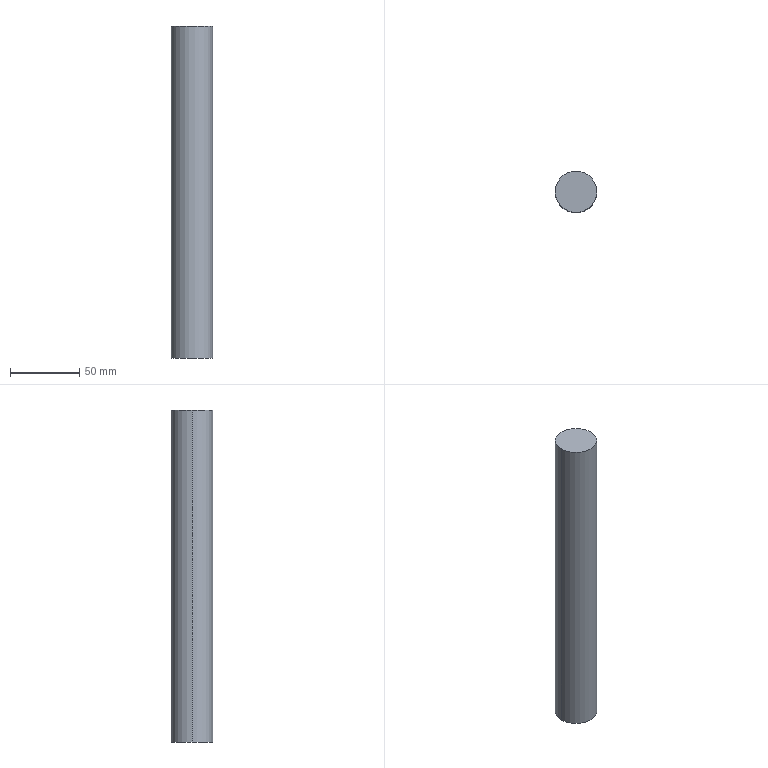Part | SolidWorks | features Extrusion 1 | 1 solid | 4 faces | box 30 x 30 x 240 mm | volume 169646 mm3 | cylinder 2 | plane 2 | commonest cylinder face diameters 30 x2
STEP:
#1=CARTESIAN_POINT('',(15.,0.,200.));
#2=VERTEX_POINT('',#1);
#3=CARTESIAN_POINT('',(-15.,0.,200.));
#4=VERTEX_POINT('',#3);
#5=CARTESIAN_POINT('',(0.,0.,200.));
#6=DIRECTION('',(0.,0.,1.));
#7=DIRECTION('',(1.,0.,0.));
#8=AXIS2_PLACEMENT_3D('',#5,#6,#7);
#9=CIRCLE('',#8,15.);
#10=EDGE_CURVE('',#2,#4,#9,.T.);
#11=ORIENTED_EDGE('',*,*,#10,.F.);
#12=CARTESIAN_POINT('',(15.,0.,-40.));
#13=VERTEX_POINT('',#12);
#14=CARTESIAN_POINT('',(15.,0.,200.));
#15=DIRECTION('',(0.,0.,-1.));
#16=VECTOR('',#15,1000.);
#17=LINE('',#14,#16);
#18=EDGE_CURVE('',#2,#13,#17,.T.);
#19=ORIENTED_EDGE('',*,*,#18,.T.);
#20=CARTESIAN_POINT('',(-15.,0.,-40.));
#21=VERTEX_POINT('',#20);
#22=CARTESIAN_POINT('',(0.,0.,-40.));
#23=DIRECTION('',(0.,0.,1.));
#24=DIRECTION('',(1.,0.,0.));
#25=AXIS2_PLACEMENT_3D('',#22,#23,#24);
#26=CIRCLE('',#25,15.);
#27=EDGE_CURVE('',#13,#21,#26,.T.);
#28=ORIENTED_EDGE('',*,*,#27,.T.);
#29=CARTESIAN_POINT('',(-15.,0.,200.));
#30=DIRECTION('',(0.,0.,-1.));
#31=VECTOR('',#30,1000.);
#32=LINE('',#29,#31);
#33=EDGE_CURVE('',#4,#21,#32,.T.);
#34=ORIENTED_EDGE('',*,*,#33,.F.);
#35=EDGE_LOOP('',(#11,#19,#28,#34));
#36=FACE_OUTER_BOUND('',#35,.T.);
#37=CARTESIAN_POINT('',(0.,0.,200.));
#38=DIRECTION('',(0.,0.,-1.));
#39=DIRECTION('',(-1.,0.,0.));
#40=AXIS2_PLACEMENT_3D('',#37,#38,#39);
#41=CYLINDRICAL_SURFACE('',#40,15.);
#42=ADVANCED_FACE('',(#36),#41,.T.);
#43=ORIENTED_EDGE('',*,*,#18,.F.);
#44=CARTESIAN_POINT('',(0.,0.,200.));
#45=DIRECTION('',(0.,0.,1.));
#46=DIRECTION('',(1.,0.,0.));
#47=AXIS2_PLACEMENT_3D('',#44,#45,#46);
#48=CIRCLE('',#47,15.);
#49=EDGE_CURVE('',#4,#2,#48,.T.);
#50=ORIENTED_EDGE('',*,*,#49,.F.);
#51=ORIENTED_EDGE('',*,*,#33,.T.);
#52=CARTESIAN_POINT('',(0.,0.,-40.));
#53=DIRECTION('',(0.,0.,1.));
#54=DIRECTION('',(1.,0.,0.));
#55=AXIS2_PLACEMENT_3D('',#52,#53,#54);
#56=CIRCLE('',#55,15.);
#57=EDGE_CURVE('',#21,#13,#56,.T.);
#58=ORIENTED_EDGE('',*,*,#57,.T.);
#59=EDGE_LOOP('',(#43,#50,#51,#58));
#60=FACE_OUTER_BOUND('',#59,.T.);
#61=CARTESIAN_POINT('',(0.,0.,200.));
#62=DIRECTION('',(0.,0.,-1.));
#63=DIRECTION('',(-1.,0.,0.));
#64=AXIS2_PLACEMENT_3D('',#61,#62,#63);
#65=CYLINDRICAL_SURFACE('',#64,15.);
#66=ADVANCED_FACE('',(#60),#65,.T.);
#67=ORIENTED_EDGE('',*,*,#49,.T.);
#68=ORIENTED_EDGE('',*,*,#10,.T.);
#69=EDGE_LOOP('',(#67,#68));
#70=FACE_OUTER_BOUND('',#69,.T.);
#71=CARTESIAN_POINT('',(0.,0.,200.));
#72=DIRECTION('',(0.,0.,1.));
#73=DIRECTION('',(1.,0.,0.));
#74=AXIS2_PLACEMENT_3D('',#71,#72,#73);
#75=PLANE('',#74);
#76=ADVANCED_FACE('',(#70),#75,.T.);
#77=ORIENTED_EDGE('',*,*,#57,.F.);
#78=ORIENTED_EDGE('',*,*,#27,.F.);
#79=EDGE_LOOP('',(#77,#78));
#80=FACE_OUTER_BOUND('',#79,.T.);
#81=CARTESIAN_POINT('',(0.,0.,-40.));
#82=DIRECTION('',(0.,0.,1.));
#83=DIRECTION('',(1.,0.,0.));
#84=AXIS2_PLACEMENT_3D('',#81,#82,#83);
#85=PLANE('',#84);
#86=ADVANCED_FACE('',(#80),#85,.F.);
#87=CLOSED_SHELL('',(#42,#66,#76,#86));
#88=MANIFOLD_SOLID_BREP('',#87);
#89=CARTESIAN_POINT('',(0.,0.,0.));
#90=DIRECTION('',(0.,0.,1.));
#91=DIRECTION('',(1.,0.,0.));
#92=AXIS2_PLACEMENT_3D('',#89,#90,#91);
#93=(LENGTH_UNIT()NAMED_UNIT(*)SI_UNIT(.MILLI.,.METRE.));
#94=UNCERTAINTY_MEASURE_WITH_UNIT(LENGTH_MEASURE(0.00001),#93,'','');
#95=(NAMED_UNIT(*)PLANE_ANGLE_UNIT()SI_UNIT($,.RADIAN.));
#96=(NAMED_UNIT(*)SI_UNIT($,.STERADIAN.)SOLID_ANGLE_UNIT());
#97=(GEOMETRIC_REPRESENTATION_CONTEXT(3)GLOBAL_UNCERTAINTY_ASSIGNED_CONTEXT((#94))GLOBAL_UNIT_ASSIGNED_CONTEXT((#93,#95,#96))REPRESENTATION_CONTEXT('',''));
#98=ADVANCED_BREP_SHAPE_REPRESENTATION('',(#88,#92),#97);